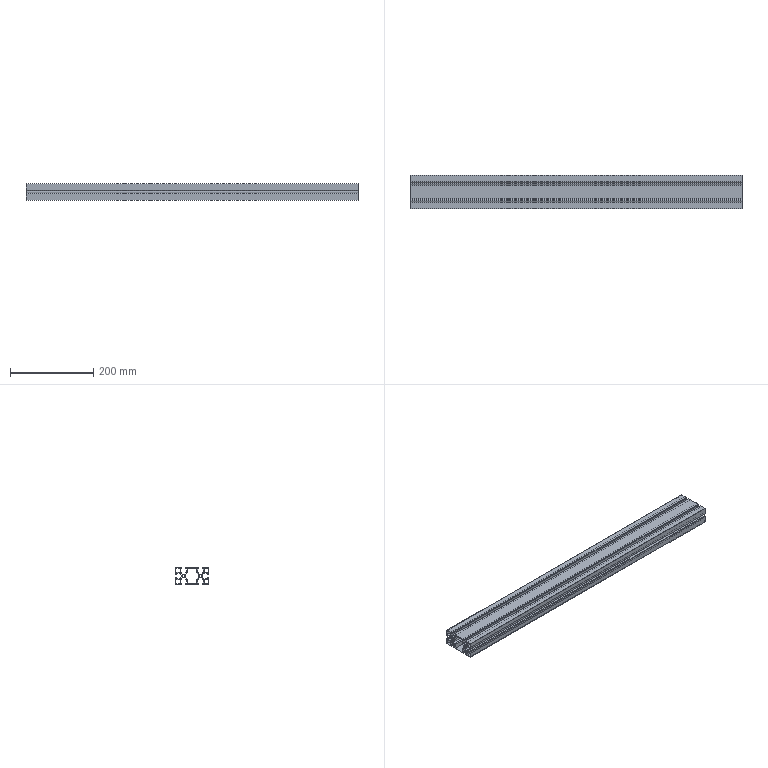Part | 1 solid | 126 faces | box 800 x 80 x 40 mm | volume 554871 mm3 | plane 110 | cylinder 16 | commonest cylinder face diameters 9.6 x10 6.6 x4 0.6 x2